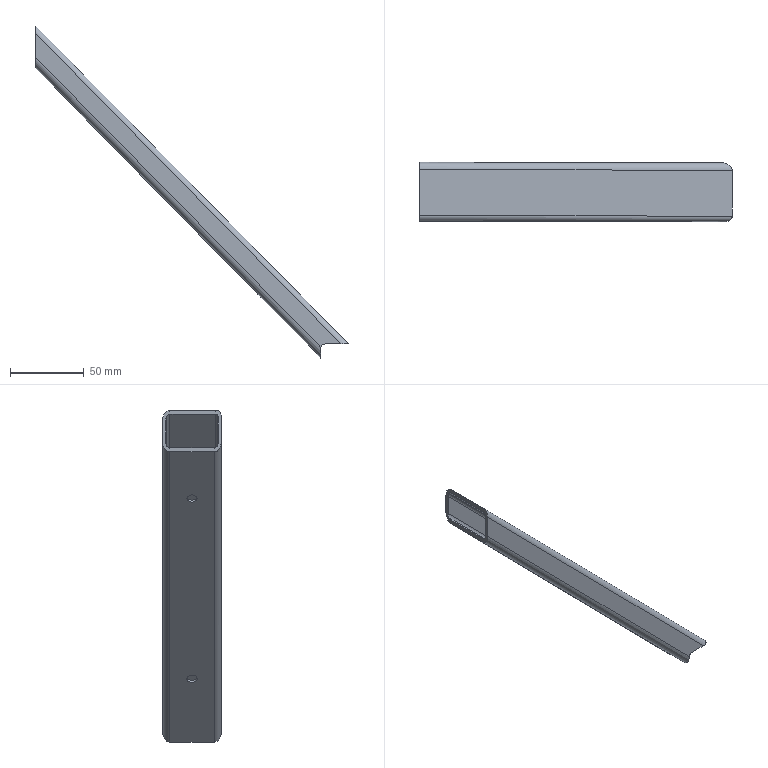Part | NX | features BREP 1 | 1 solid | 31 faces | box 212.69 x 40 x 225.842 mm | volume 60669 mm3 | cylinder 18 | plane 13 | commonest cylinder face diameters 6 x8 7 x4 10 x3 3.502 x2 7.502 x1
STEP:
#1=CARTESIAN_POINT('',(2103.23,-625.419,1266.938));
#2=VERTEX_POINT('',#1);
#3=CARTESIAN_POINT('',(1890.54,-625.419,1483.221));
#4=VERTEX_POINT('',#3);
#5=CARTESIAN_POINT('',(1990.472,-625.419,1381.601));
#6=DIRECTION('',(-0.7012,0.,0.713));
#7=VECTOR('',#6,1000.);
#8=LINE('',#5,#7);
#9=EDGE_CURVE('',#2,#4,#8,.T.);
#10=ORIENTED_EDGE('',*,*,#9,.F.);
#11=CARTESIAN_POINT('',(2103.23,-594.17,1266.938));
#12=VERTEX_POINT('',#11);
#13=CARTESIAN_POINT('',(2103.23,-609.794,1266.938));
#14=DIRECTION('',(0.,-1.,0.));
#15=VECTOR('',#14,1000.);
#16=LINE('',#13,#15);
#17=EDGE_CURVE('',#12,#2,#16,.T.);
#18=ORIENTED_EDGE('',*,*,#17,.F.);
#19=CARTESIAN_POINT('',(1890.54,-594.17,1483.221));
#20=VERTEX_POINT('',#19);
#21=CARTESIAN_POINT('',(1990.472,-594.17,1381.601));
#22=DIRECTION('',(-0.7012,0.,0.713));
#23=VECTOR('',#22,1000.);
#24=LINE('',#21,#23);
#25=EDGE_CURVE('',#12,#20,#24,.T.);
#26=ORIENTED_EDGE('',*,*,#25,.T.);
#27=CARTESIAN_POINT('',(1890.54,-625.419,1483.221));
#28=CARTESIAN_POINT('',(1890.54,-619.169,1483.221));
#29=CARTESIAN_POINT('',(1890.54,-612.919,1483.221));
#30=CARTESIAN_POINT('',(1890.54,-606.67,1483.221));
#31=CARTESIAN_POINT('',(1890.54,-600.42,1483.221));
#32=CARTESIAN_POINT('',(1890.54,-594.17,1483.221));
#33=B_SPLINE_CURVE_WITH_KNOTS('',5,(#27,#28,#29,#30,#31,#32),.UNSPECIFIED.,.F.,.F.,(6,6),(417.921,449.17),.UNSPECIFIED.);
#34=EDGE_CURVE('',#4,#20,#33,.T.);
#35=ORIENTED_EDGE('',*,*,#34,.F.);
#36=EDGE_LOOP('',(#10,#18,#26,#35));
#37=FACE_BOUND('',#36,.T.);
#38=CARTESIAN_POINT('',(2067.213,-625.419,1303.563));
#39=DIRECTION('',(0.713,0.,0.7012));
#40=DIRECTION('',(0.,1.,0.));
#41=AXIS2_PLACEMENT_3D('',#38,#39,#40);
#42=PLANE('',#41);
#43=ADVANCED_FACE('',(#37),#42,.T.);
#44=CARTESIAN_POINT('',(2097.968,-629.17,1266.938));
#45=VERTEX_POINT('',#44);
#46=CARTESIAN_POINT('',(2087.579,-629.17,1266.938));
#47=VERTEX_POINT('',#46);
#48=CARTESIAN_POINT('',(2092.774,-629.17,1266.938));
#49=DIRECTION('',(-1.,0.,0.));
#50=VECTOR('',#49,1000.);
#51=LINE('',#48,#50);
#52=EDGE_CURVE('',#45,#47,#51,.T.);
#53=ORIENTED_EDGE('',*,*,#52,.T.);
#54=CARTESIAN_POINT('',(2087.579,-627.17,1266.938));
#55=VERTEX_POINT('',#54);
#56=CARTESIAN_POINT('',(2087.579,-728.755,1266.938));
#57=DIRECTION('',(0.,1.,0.));
#58=VECTOR('',#57,1000.);
#59=LINE('',#56,#58);
#60=EDGE_CURVE('',#47,#55,#59,.T.);
#61=ORIENTED_EDGE('',*,*,#60,.T.);
#62=CARTESIAN_POINT('',(2097.968,-627.17,1266.938));
#63=VERTEX_POINT('',#62);
#64=CARTESIAN_POINT('',(2092.774,-627.17,1266.938));
#65=DIRECTION('',(-1.,0.,0.));
#66=VECTOR('',#65,1000.);
#67=LINE('',#64,#66);
#68=EDGE_CURVE('',#63,#55,#67,.T.);
#69=ORIENTED_EDGE('',*,*,#68,.F.);
#70=CARTESIAN_POINT('',(2099.705,-626.657,1266.938));
#71=VERTEX_POINT('',#70);
#72=CARTESIAN_POINT('',(2097.968,-627.17,1266.938));
#73=CARTESIAN_POINT('',(2098.602,-627.17,1266.938));
#74=CARTESIAN_POINT('',(2099.227,-626.998,1266.938));
#75=CARTESIAN_POINT('',(2099.705,-626.657,1266.938));
#76=B_SPLINE_CURVE_WITH_KNOTS('',3,(#72,#73,#74,#75),.UNSPECIFIED.,.F.,.F.,(4,4),(0.,1.),.UNSPECIFIED.);
#77=EDGE_CURVE('',#71,#63,#76,.F.);
#78=ORIENTED_EDGE('',*,*,#77,.F.);
#79=CARTESIAN_POINT('',(2100.425,-625.419,1266.938));
#80=VERTEX_POINT('',#79);
#81=CARTESIAN_POINT('',(2099.705,-626.657,1266.938));
#82=CARTESIAN_POINT('',(2100.15,-626.34,1266.938));
#83=CARTESIAN_POINT('',(2100.425,-625.899,1266.938));
#84=CARTESIAN_POINT('',(2100.425,-625.419,1266.938));
#85=B_SPLINE_CURVE_WITH_KNOTS('',3,(#81,#82,#83,#84),.UNSPECIFIED.,.F.,.F.,(4,4),(0.,1.),.UNSPECIFIED.);
#86=EDGE_CURVE('',#80,#71,#85,.F.);
#87=ORIENTED_EDGE('',*,*,#86,.F.);
#88=CARTESIAN_POINT('',(2100.425,-594.17,1266.938));
#89=VERTEX_POINT('',#88);
#90=CARTESIAN_POINT('',(2100.425,-609.794,1266.938));
#91=DIRECTION('',(0.,1.,0.));
#92=VECTOR('',#91,1000.);
#93=LINE('',#90,#92);
#94=EDGE_CURVE('',#80,#89,#93,.T.);
#95=ORIENTED_EDGE('',*,*,#94,.T.);
#96=CARTESIAN_POINT('',(2099.192,-592.049,1266.938));
#97=VERTEX_POINT('',#96);
#98=CARTESIAN_POINT('',(2100.425,-594.17,1266.938));
#99=CARTESIAN_POINT('',(2100.425,-593.338,1266.938));
#100=CARTESIAN_POINT('',(2099.922,-592.569,1266.938));
#101=CARTESIAN_POINT('',(2099.192,-592.049,1266.938));
#102=B_SPLINE_CURVE_WITH_KNOTS('',3,(#98,#99,#100,#101),.UNSPECIFIED.,.F.,.F.,(4,4),(0.,1.),.UNSPECIFIED.);
#103=EDGE_CURVE('',#89,#97,#102,.T.);
#104=ORIENTED_EDGE('',*,*,#103,.T.);
#105=CARTESIAN_POINT('',(2096.217,-591.17,1266.938));
#106=VERTEX_POINT('',#105);
#107=CARTESIAN_POINT('',(2099.192,-592.049,1266.938));
#108=CARTESIAN_POINT('',(2098.37,-591.463,1266.938));
#109=CARTESIAN_POINT('',(2097.283,-591.17,1266.938));
#110=CARTESIAN_POINT('',(2096.217,-591.17,1266.938));
#111=B_SPLINE_CURVE_WITH_KNOTS('',3,(#107,#108,#109,#110),.UNSPECIFIED.,.F.,.F.,(4,4),(0.,1.),.UNSPECIFIED.);
#112=EDGE_CURVE('',#97,#106,#111,.T.);
#113=ORIENTED_EDGE('',*,*,#112,.T.);
#114=CARTESIAN_POINT('',(2087.579,-591.17,1266.938));
#115=VERTEX_POINT('',#114);
#116=CARTESIAN_POINT('',(2091.898,-591.17,1266.938));
#117=DIRECTION('',(-1.,0.,0.));
#118=VECTOR('',#117,1000.);
#119=LINE('',#116,#118);
#120=EDGE_CURVE('',#106,#115,#119,.T.);
#121=ORIENTED_EDGE('',*,*,#120,.T.);
#122=CARTESIAN_POINT('',(2087.579,-589.17,1266.938));
#123=VERTEX_POINT('',#122);
#124=CARTESIAN_POINT('',(2087.579,-708.755,1266.938));
#125=DIRECTION('',(0.,1.,0.));
#126=VECTOR('',#125,1000.);
#127=LINE('',#124,#126);
#128=EDGE_CURVE('',#115,#123,#127,.T.);
#129=ORIENTED_EDGE('',*,*,#128,.T.);
#130=CARTESIAN_POINT('',(2096.217,-589.17,1266.938));
#131=VERTEX_POINT('',#130);
#132=CARTESIAN_POINT('',(2091.898,-589.17,1266.938));
#133=DIRECTION('',(-1.,0.,0.));
#134=VECTOR('',#133,1000.);
#135=LINE('',#132,#134);
#136=EDGE_CURVE('',#131,#123,#135,.T.);
#137=ORIENTED_EDGE('',*,*,#136,.F.);
#138=CARTESIAN_POINT('',(2096.217,-589.17,1266.938));
#139=CARTESIAN_POINT('',(2097.807,-589.17,1266.938));
#140=CARTESIAN_POINT('',(2100.201,-589.72,1266.938));
#141=CARTESIAN_POINT('',(2102.668,-591.822,1266.938));
#142=CARTESIAN_POINT('',(2103.23,-593.382,1266.938));
#143=CARTESIAN_POINT('',(2103.23,-594.17,1266.938));
#144=B_SPLINE_CURVE_WITH_KNOTS('',3,(#138,#139,#140,#141,#142,#143),.UNSPECIFIED.,.F.,.F.,(4,1,1,4),(0.,0.5,0.75,1.),.UNSPECIFIED.);
#145=EDGE_CURVE('',#12,#131,#144,.F.);
#146=ORIENTED_EDGE('',*,*,#145,.F.);
#147=ORIENTED_EDGE('',*,*,#17,.T.);
#148=CARTESIAN_POINT('',(2103.23,-625.419,1266.938));
#149=CARTESIAN_POINT('',(2103.23,-625.838,1266.938));
#150=CARTESIAN_POINT('',(2103.147,-626.257,1266.938));
#151=CARTESIAN_POINT('',(2102.983,-626.653,1266.938));
#152=CARTESIAN_POINT('',(2102.411,-627.575,1266.938));
#153=CARTESIAN_POINT('',(2101.543,-628.249,1266.938));
#154=CARTESIAN_POINT('',(2100.956,-628.566,1266.938));
#155=CARTESIAN_POINT('',(2100.01,-628.927,1266.938));
#156=CARTESIAN_POINT('',(2099.019,-629.107,1266.938));
#157=CARTESIAN_POINT('',(2098.67,-629.149,1266.938));
#158=CARTESIAN_POINT('',(2098.319,-629.17,1266.938));
#159=CARTESIAN_POINT('',(2097.968,-629.17,1266.938));
#160=B_SPLINE_CURVE_WITH_KNOTS('',5,(#148,#149,#150,#151,#152,#153,#154,#155,#156,#157,#158,#159),.UNSPECIFIED.,.F.,.F.,(6,3,3,6),(0.,2.975,7.619,10.108),.UNSPECIFIED.);
#161=EDGE_CURVE('',#2,#45,#160,.T.);
#162=ORIENTED_EDGE('',*,*,#161,.T.);
#163=EDGE_LOOP('',(#53,#61,#69,#78,#87,#95,#104,#113,#121,#129,#137,#146,#147,#162));
#164=FACE_BOUND('',#163,.T.);
#165=CARTESIAN_POINT('',(2104.579,-414.17,1266.938));
#166=DIRECTION('',(0.,0.,1.));
#167=DIRECTION('',(-1.,0.,0.));
#168=AXIS2_PLACEMENT_3D('',#165,#166,#167);
#169=PLANE('',#168);
#170=ADVANCED_FACE('',(#164),#169,.F.);
#171=CARTESIAN_POINT('',(1890.54,-627.17,1477.871));
#172=VERTEX_POINT('',#171);
#173=CARTESIAN_POINT('',(1987.797,-627.17,1378.971));
#174=DIRECTION('',(-0.7012,0.,0.713));
#175=VECTOR('',#174,1000.);
#176=LINE('',#173,#175);
#177=EDGE_CURVE('',#63,#172,#176,.T.);
#178=ORIENTED_EDGE('',*,*,#177,.F.);
#179=ORIENTED_EDGE('',*,*,#68,.T.);
#180=CARTESIAN_POINT('',(2084.625,-627.17,1264.464));
#181=VERTEX_POINT('',#180);
#182=CARTESIAN_POINT('',(2087.579,-627.17,1263.938));
#183=DIRECTION('',(0.,1.,0.));
#184=DIRECTION('',(1.,0.,0.));
#185=AXIS2_PLACEMENT_3D('',#182,#183,#184);
#186=CIRCLE('',#185,3.);
#187=EDGE_CURVE('',#181,#55,#186,.T.);
#188=ORIENTED_EDGE('',*,*,#187,.F.);
#189=CARTESIAN_POINT('',(1890.54,-627.17,1461.828));
#190=VERTEX_POINT('',#189);
#191=CARTESIAN_POINT('',(1979.777,-627.17,1371.084));
#192=DIRECTION('',(-0.7012,0.,0.713));
#193=VECTOR('',#192,1000.);
#194=LINE('',#191,#193);
#195=EDGE_CURVE('',#181,#190,#194,.T.);
#196=ORIENTED_EDGE('',*,*,#195,.T.);
#197=CARTESIAN_POINT('',(1890.54,-627.17,1469.85));
#198=DIRECTION('',(0.,0.,-1.));
#199=VECTOR('',#198,1000.);
#200=LINE('',#197,#199);
#201=EDGE_CURVE('',#172,#190,#200,.T.);
#202=ORIENTED_EDGE('',*,*,#201,.F.);
#203=EDGE_LOOP('',(#178,#179,#188,#196,#202));
#204=FACE_BOUND('',#203,.T.);
#205=CARTESIAN_POINT('',(1839.262,-627.17,1468.228));
#206=DIRECTION('',(0.,-1.,0.));
#207=DIRECTION('',(-0.008377,0.,-1.));
#208=AXIS2_PLACEMENT_3D('',#205,#206,#207);
#209=PLANE('',#208);
#210=ADVANCED_FACE('',(#204),#209,.F.);
#211=ORIENTED_EDGE('',*,*,#77,.T.);
#212=ORIENTED_EDGE('',*,*,#177,.T.);
#213=CARTESIAN_POINT('',(1890.54,-626.657,1479.637));
#214=VERTEX_POINT('',#213);
#215=CARTESIAN_POINT('',(1890.54,-626.657,1479.637));
#216=CARTESIAN_POINT('',(1890.54,-626.995,1479.156));
#217=CARTESIAN_POINT('',(1890.54,-627.17,1478.515));
#218=CARTESIAN_POINT('',(1890.54,-627.17,1477.871));
#219=B_SPLINE_CURVE_WITH_KNOTS('',3,(#215,#216,#217,#218),.UNSPECIFIED.,.F.,.F.,(4,4),(0.,1.),.UNSPECIFIED.);
#220=EDGE_CURVE('',#214,#172,#219,.T.);
#221=ORIENTED_EDGE('',*,*,#220,.F.);
#222=CARTESIAN_POINT('',(1988.68,-626.657,1379.839));
#223=DIRECTION('',(-0.7012,0.,0.713));
#224=VECTOR('',#223,1000.);
#225=LINE('',#222,#224);
#226=EDGE_CURVE('',#71,#214,#225,.T.);
#227=ORIENTED_EDGE('',*,*,#226,.F.);
#228=EDGE_LOOP('',(#211,#212,#221,#227));
#229=FACE_BOUND('',#228,.T.);
#230=CARTESIAN_POINT('',(1987.797,-625.419,1378.971));
#231=DIRECTION('',(-0.7012,0.,0.713));
#232=DIRECTION('',(-0.5042,0.7071,-0.4958));
#233=AXIS2_PLACEMENT_3D('',#230,#231,#232);
#234=CYLINDRICAL_SURFACE('',#233,1.751);
#235=ADVANCED_FACE('',(#229),#234,.F.);
#236=CARTESIAN_POINT('',(1890.54,-625.419,1480.369));
#237=VERTEX_POINT('',#236);
#238=CARTESIAN_POINT('',(1890.54,-625.419,1480.369));
#239=CARTESIAN_POINT('',(1890.54,-625.902,1480.369));
#240=CARTESIAN_POINT('',(1890.54,-626.341,1480.088));
#241=CARTESIAN_POINT('',(1890.54,-626.657,1479.637));
#242=B_SPLINE_CURVE_WITH_KNOTS('',3,(#238,#239,#240,#241),.UNSPECIFIED.,.F.,.F.,(4,4),(0.,1.),.UNSPECIFIED.);
#243=EDGE_CURVE('',#237,#214,#242,.T.);
#244=ORIENTED_EDGE('',*,*,#243,.F.);
#245=CARTESIAN_POINT('',(1995.482,-625.419,1373.654));
#246=DIRECTION('',(-0.7012,0.,0.713));
#247=VECTOR('',#246,1000.);
#248=LINE('',#245,#247);
#249=EDGE_CURVE('',#80,#237,#248,.T.);
#250=ORIENTED_EDGE('',*,*,#249,.F.);
#251=ORIENTED_EDGE('',*,*,#86,.T.);
#252=ORIENTED_EDGE('',*,*,#226,.T.);
#253=EDGE_LOOP('',(#244,#250,#251,#252));
#254=FACE_BOUND('',#253,.T.);
#255=CARTESIAN_POINT('',(1987.797,-625.419,1378.971));
#256=DIRECTION('',(-0.7012,0.,0.713));
#257=DIRECTION('',(0.5042,-0.7071,0.4958));
#258=AXIS2_PLACEMENT_3D('',#255,#256,#257);
#259=CYLINDRICAL_SURFACE('',#258,1.751);
#260=ADVANCED_FACE('',(#254),#259,.F.);
#261=CARTESIAN_POINT('',(1890.54,-594.17,1480.369));
#262=VERTEX_POINT('',#261);
#263=CARTESIAN_POINT('',(1890.54,-609.794,1480.369));
#264=DIRECTION('',(0.,1.,0.));
#265=VECTOR('',#264,1000.);
#266=LINE('',#263,#265);
#267=EDGE_CURVE('',#237,#262,#266,.T.);
#268=ORIENTED_EDGE('',*,*,#267,.T.);
#269=CARTESIAN_POINT('',(1989.046,-594.17,1380.199));
#270=DIRECTION('',(-0.7012,0.,0.713));
#271=VECTOR('',#270,1000.);
#272=LINE('',#269,#271);
#273=EDGE_CURVE('',#89,#262,#272,.T.);
#274=ORIENTED_EDGE('',*,*,#273,.F.);
#275=ORIENTED_EDGE('',*,*,#94,.F.);
#276=ORIENTED_EDGE('',*,*,#249,.T.);
#277=EDGE_LOOP('',(#268,#274,#275,#276));
#278=FACE_BOUND('',#277,.T.);
#279=CARTESIAN_POINT('',(2065.787,-625.419,1302.16));
#280=DIRECTION('',(0.713,0.,0.7012));
#281=DIRECTION('',(0.,1.,0.));
#282=AXIS2_PLACEMENT_3D('',#279,#280,#281);
#283=PLANE('',#282);
#284=ADVANCED_FACE('',(#278),#283,.F.);
#285=ORIENTED_EDGE('',*,*,#103,.F.);
#286=ORIENTED_EDGE('',*,*,#273,.T.);
#287=CARTESIAN_POINT('',(1890.54,-592.049,1479.116));
#288=VERTEX_POINT('',#287);
#289=CARTESIAN_POINT('',(1890.54,-594.17,1480.369));
#290=CARTESIAN_POINT('',(1890.54,-593.953,1480.369));
#291=CARTESIAN_POINT('',(1890.54,-593.737,1480.341));
#292=CARTESIAN_POINT('',(1890.54,-593.524,1480.285));
#293=CARTESIAN_POINT('',(1890.54,-593.051,1480.097));
#294=CARTESIAN_POINT('',(1890.54,-592.631,1479.792));
#295=CARTESIAN_POINT('',(1890.54,-592.414,1479.588));
#296=CARTESIAN_POINT('',(1890.54,-592.22,1479.361));
#297=CARTESIAN_POINT('',(1890.54,-592.049,1479.116));
#298=B_SPLINE_CURVE_WITH_KNOTS('',5,(#289,#290,#291,#292,#293,#294,#295,#296,#297),.UNSPECIFIED.,.F.,.F.,(6,3,6),(0.,1.603,3.714),.UNSPECIFIED.);
#299=EDGE_CURVE('',#262,#288,#298,.T.);
#300=ORIENTED_EDGE('',*,*,#299,.T.);
#301=CARTESIAN_POINT('',(1988.419,-592.049,1379.583));
#302=DIRECTION('',(-0.7012,0.,0.713));
#303=VECTOR('',#302,1000.);
#304=LINE('',#301,#303);
#305=EDGE_CURVE('',#97,#288,#304,.T.);
#306=ORIENTED_EDGE('',*,*,#305,.F.);
#307=EDGE_LOOP('',(#285,#286,#300,#306));
#308=FACE_BOUND('',#307,.T.);
#309=CARTESIAN_POINT('',(1986.907,-594.17,1378.095));
#310=DIRECTION('',(-0.7012,0.,0.713));
#311=DIRECTION('',(-0.5042,-0.7071,-0.4958));
#312=AXIS2_PLACEMENT_3D('',#309,#310,#311);
#313=CYLINDRICAL_SURFACE('',#312,3.);
#314=ADVANCED_FACE('',(#308),#313,.F.);
#315=CARTESIAN_POINT('',(1890.54,-591.17,1476.09));
#316=VERTEX_POINT('',#315);
#317=CARTESIAN_POINT('',(1890.54,-592.049,1479.116));
#318=CARTESIAN_POINT('',(1890.54,-592.02,1479.075));
#319=CARTESIAN_POINT('',(1890.54,-591.992,1479.033));
#320=CARTESIAN_POINT('',(1890.54,-591.964,1478.991));
#321=CARTESIAN_POINT('',(1890.54,-591.706,1478.583));
#322=CARTESIAN_POINT('',(1890.54,-591.504,1478.135));
#323=CARTESIAN_POINT('',(1890.54,-591.368,1477.715));
#324=CARTESIAN_POINT('',(1890.54,-591.239,1477.135));
#325=CARTESIAN_POINT('',(1890.54,-591.184,1476.545));
#326=CARTESIAN_POINT('',(1890.54,-591.175,1476.393));
#327=CARTESIAN_POINT('',(1890.54,-591.17,1476.242));
#328=CARTESIAN_POINT('',(1890.54,-591.17,1476.09));
#329=B_SPLINE_CURVE_WITH_KNOTS('',5,(#317,#318,#319,#320,#321,#322,#323,#324,#325,#326,#327,#328),.UNSPECIFIED.,.F.,.F.,(6,3,3,6),(3.714,4.069,7.114,8.159),.UNSPECIFIED.);
#330=EDGE_CURVE('',#288,#316,#329,.T.);
#331=ORIENTED_EDGE('',*,*,#330,.T.);
#332=CARTESIAN_POINT('',(1993.378,-591.17,1371.514));
#333=DIRECTION('',(-0.7012,0.,0.713));
#334=VECTOR('',#333,1000.);
#335=LINE('',#332,#334);
#336=EDGE_CURVE('',#106,#316,#335,.T.);
#337=ORIENTED_EDGE('',*,*,#336,.F.);
#338=ORIENTED_EDGE('',*,*,#112,.F.);
#339=ORIENTED_EDGE('',*,*,#305,.T.);
#340=EDGE_LOOP('',(#331,#337,#338,#339));
#341=FACE_BOUND('',#340,.T.);
#342=CARTESIAN_POINT('',(1986.907,-594.17,1378.095));
#343=DIRECTION('',(-0.7012,0.,0.713));
#344=DIRECTION('',(0.5042,0.7071,0.4958));
#345=AXIS2_PLACEMENT_3D('',#342,#343,#344);
#346=CYLINDRICAL_SURFACE('',#345,3.);
#347=ADVANCED_FACE('',(#341),#346,.F.);
#348=CARTESIAN_POINT('',(2084.625,-591.17,1264.464));
#349=VERTEX_POINT('',#348);
#350=CARTESIAN_POINT('',(2087.579,-591.17,1263.938));
#351=DIRECTION('',(0.,1.,0.));
#352=DIRECTION('',(1.,0.,0.));
#353=AXIS2_PLACEMENT_3D('',#350,#351,#352);
#354=CIRCLE('',#353,3.);
#355=EDGE_CURVE('',#349,#115,#354,.T.);
#356=ORIENTED_EDGE('',*,*,#355,.T.);
#357=ORIENTED_EDGE('',*,*,#120,.F.);
#358=ORIENTED_EDGE('',*,*,#336,.T.);
#359=CARTESIAN_POINT('',(1890.54,-591.17,1461.828));
#360=VERTEX_POINT('',#359);
#361=CARTESIAN_POINT('',(1890.54,-591.17,1468.959));
#362=DIRECTION('',(0.,0.,-1.));
#363=VECTOR('',#362,1000.);
#364=LINE('',#361,#363);
#365=EDGE_CURVE('',#316,#360,#364,.T.);
#366=ORIENTED_EDGE('',*,*,#365,.T.);
#367=CARTESIAN_POINT('',(1979.777,-591.17,1371.084));
#368=DIRECTION('',(-0.7012,0.,0.713));
#369=VECTOR('',#368,1000.);
#370=LINE('',#367,#369);
#371=EDGE_CURVE('',#349,#360,#370,.T.);
#372=ORIENTED_EDGE('',*,*,#371,.F.);
#373=EDGE_LOOP('',(#356,#357,#358,#366,#372));
#374=FACE_BOUND('',#373,.T.);
#375=CARTESIAN_POINT('',(1839.168,-591.17,1456.98));
#376=DIRECTION('',(0.,1.,0.));
#377=DIRECTION('',(0.008377,0.,1.));
#378=AXIS2_PLACEMENT_3D('',#375,#376,#377);
#379=PLANE('',#378);
#380=ADVANCED_FACE('',(#374),#379,.F.);
#381=CARTESIAN_POINT('',(2084.625,-589.17,1264.464));
#382=VERTEX_POINT('',#381);
#383=CARTESIAN_POINT('',(1890.54,-589.17,1461.828));
#384=VERTEX_POINT('',#383);
#385=CARTESIAN_POINT('',(1979.777,-589.17,1371.084));
#386=DIRECTION('',(-0.7012,0.,0.713));
#387=VECTOR('',#386,1000.);
#388=LINE('',#385,#387);
#389=EDGE_CURVE('',#382,#384,#388,.T.);
#390=ORIENTED_EDGE('',*,*,#389,.T.);
#391=CARTESIAN_POINT('',(1890.54,-589.17,1476.09));
#392=VERTEX_POINT('',#391);
#393=CARTESIAN_POINT('',(1890.54,-589.17,1468.959));
#394=DIRECTION('',(0.,0.,-1.));
#395=VECTOR('',#394,1000.);
#396=LINE('',#393,#395);
#397=EDGE_CURVE('',#392,#384,#396,.T.);
#398=ORIENTED_EDGE('',*,*,#397,.F.);
#399=CARTESIAN_POINT('',(1986.907,-589.17,1378.095));
#400=DIRECTION('',(-0.7012,0.,0.713));
#401=VECTOR('',#400,1000.);
#402=LINE('',#399,#401);
#403=EDGE_CURVE('',#131,#392,#402,.T.);
#404=ORIENTED_EDGE('',*,*,#403,.F.);
#405=ORIENTED_EDGE('',*,*,#136,.T.);
#406=CARTESIAN_POINT('',(2087.579,-589.17,1263.938));
#407=DIRECTION('',(0.,1.,0.));
#408=DIRECTION('',(1.,0.,0.));
#409=AXIS2_PLACEMENT_3D('',#406,#407,#408);
#410=CIRCLE('',#409,3.);
#411=EDGE_CURVE('',#382,#123,#410,.T.);
#412=ORIENTED_EDGE('',*,*,#411,.F.);
#413=EDGE_LOOP('',(#390,#398,#404,#405,#412));
#414=FACE_BOUND('',#413,.T.);
#415=CARTESIAN_POINT('',(1839.168,-589.17,1456.98));
#416=DIRECTION('',(0.,1.,0.));
#417=DIRECTION('',(0.008377,0.,1.));
#418=AXIS2_PLACEMENT_3D('',#415,#416,#417);
#419=PLANE('',#418);
#420=ADVANCED_FACE('',(#414),#419,.T.);
#421=ORIENTED_EDGE('',*,*,#403,.T.);
#422=CARTESIAN_POINT('',(1890.54,-592.854,1482.97));
#423=VERTEX_POINT('',#422);
#424=CARTESIAN_POINT('',(1890.54,-592.854,1482.97));
#425=CARTESIAN_POINT('',(1890.54,-592.47,1482.82));
#426=CARTESIAN_POINT('',(1890.54,-592.105,1482.62));
#427=CARTESIAN_POINT('',(1890.54,-591.767,1482.377));
#428=CARTESIAN_POINT('',(1890.54,-591.081,1481.767));
#429=CARTESIAN_POINT('',(1890.54,-590.53,1481.03));
#430=CARTESIAN_POINT('',(1890.54,-590.267,1480.599));
#431=CARTESIAN_POINT('',(1890.54,-589.711,1479.488));
#432=CARTESIAN_POINT('',(1890.54,-589.37,1478.29));
#433=CARTESIAN_POINT('',(1890.54,-589.237,1477.562));
#434=CARTESIAN_POINT('',(1890.54,-589.17,1476.826));
#435=CARTESIAN_POINT('',(1890.54,-589.17,1476.09));
#436=B_SPLINE_CURVE_WITH_KNOTS('',5,(#424,#425,#426,#427,#428,#429,#430,#431,#432,#433,#434,#435),.UNSPECIFIED.,.F.,.F.,(6,3,3,6),(0.,2.919,6.476,11.688),.UNSPECIFIED.);
#437=EDGE_CURVE('',#423,#392,#436,.T.);
#438=ORIENTED_EDGE('',*,*,#437,.F.);
#439=CARTESIAN_POINT('',(1890.54,-594.17,1483.221));
#440=CARTESIAN_POINT('',(1890.54,-593.723,1483.221));
#441=CARTESIAN_POINT('',(1890.54,-593.285,1483.138));
#442=CARTESIAN_POINT('',(1890.54,-592.854,1482.97));
#443=B_SPLINE_CURVE_WITH_KNOTS('',3,(#439,#440,#441,#442),.UNSPECIFIED.,.F.,.F.,(4,4),(0.,1.),.UNSPECIFIED.);
#444=EDGE_CURVE('',#20,#423,#443,.T.);
#445=ORIENTED_EDGE('',*,*,#444,.F.);
#446=ORIENTED_EDGE('',*,*,#25,.F.);
#447=ORIENTED_EDGE('',*,*,#145,.T.);
#448=EDGE_LOOP('',(#421,#438,#445,#446,#447));
#449=FACE_BOUND('',#448,.T.);
#450=CARTESIAN_POINT('',(1986.907,-594.17,1378.095));
#451=DIRECTION('',(-0.7012,0.,0.713));
#452=DIRECTION('',(0.713,0.,0.7012));
#453=AXIS2_PLACEMENT_3D('',#450,#451,#452);
#454=CYLINDRICAL_SURFACE('',#453,5.);
#455=ADVANCED_FACE('',(#449),#454,.T.);
#456=CARTESIAN_POINT('',(1890.54,-594.17,1482.97));
#457=VERTEX_POINT('',#456);
#458=CARTESIAN_POINT('',(1890.54,-594.17,1482.97));
#459=CARTESIAN_POINT('',(1890.54,-594.17,1483.221));
#460=B_SPLINE_CURVE_WITH_KNOTS('',1,(#458,#459),.UNSPECIFIED.,.F.,.F.,(2,2),(0.,0.2516),.UNSPECIFIED.);
#461=EDGE_CURVE('',#457,#20,#460,.T.);
#462=ORIENTED_EDGE('',*,*,#461,.T.);
#463=ORIENTED_EDGE('',*,*,#444,.T.);
#464=CARTESIAN_POINT('',(1890.54,-593.512,1482.97));
#465=DIRECTION('',(0.,1.,0.));
#466=VECTOR('',#465,1000.);
#467=LINE('',#464,#466);
#468=EDGE_CURVE('',#457,#423,#467,.T.);
#469=ORIENTED_EDGE('',*,*,#468,.F.);
#470=EDGE_LOOP('',(#462,#463,#469));
#471=FACE_BOUND('',#470,.T.);
#472=CARTESIAN_POINT('',(1890.54,-394.17,1483.14));
#473=DIRECTION('',(1.,0.,0.));
#474=DIRECTION('',(0.,0.,-1.));
#475=AXIS2_PLACEMENT_3D('',#472,#473,#474);
#476=PLANE('',#475);
#477=ADVANCED_FACE('',(#471),#476,.F.);
#478=CARTESIAN_POINT('',(1890.54,-626.556,1482.97));
#479=VERTEX_POINT('',#478);
#480=CARTESIAN_POINT('',(1890.54,-626.556,1482.97));
#481=CARTESIAN_POINT('',(1890.54,-626.187,1483.137));
#482=CARTESIAN_POINT('',(1890.54,-625.803,1483.221));
#483=CARTESIAN_POINT('',(1890.54,-625.419,1483.221));
#484=B_SPLINE_CURVE_WITH_KNOTS('',3,(#480,#481,#482,#483),.UNSPECIFIED.,.F.,.F.,(4,4),(0.,1.),.UNSPECIFIED.);
#485=EDGE_CURVE('',#4,#479,#484,.F.);
#486=ORIENTED_EDGE('',*,*,#485,.F.);
#487=ORIENTED_EDGE('',*,*,#34,.T.);
#488=ORIENTED_EDGE('',*,*,#461,.F.);
#489=CARTESIAN_POINT('',(1890.54,-610.363,1482.97));
#490=DIRECTION('',(0.,1.,0.));
#491=VECTOR('',#490,1000.);
#492=LINE('',#489,#491);
#493=EDGE_CURVE('',#479,#457,#492,.T.);
#494=ORIENTED_EDGE('',*,*,#493,.F.);
#495=EDGE_LOOP('',(#486,#487,#488,#494));
#496=FACE_BOUND('',#495,.T.);
#497=CARTESIAN_POINT('',(1890.54,-414.17,1483.14));
#498=DIRECTION('',(1.,0.,0.));
#499=DIRECTION('',(0.,0.,-1.));
#500=AXIS2_PLACEMENT_3D('',#497,#498,#499);
#501=PLANE('',#500);
#502=ADVANCED_FACE('',(#496),#501,.F.);
#503=ORIENTED_EDGE('',*,*,#9,.T.);
#504=ORIENTED_EDGE('',*,*,#485,.T.);
#505=CARTESIAN_POINT('',(1890.54,-629.17,1477.871));
#506=VERTEX_POINT('',#505);
#507=CARTESIAN_POINT('',(1890.54,-626.556,1482.97));
#508=CARTESIAN_POINT('',(1890.54,-626.8,1482.859));
#509=CARTESIAN_POINT('',(1890.54,-627.032,1482.721));
#510=CARTESIAN_POINT('',(1890.54,-627.25,1482.56));
#511=CARTESIAN_POINT('',(1890.54,-627.779,1482.088));
#512=CARTESIAN_POINT('',(1890.54,-628.2,1481.514));
#513=CARTESIAN_POINT('',(1890.54,-628.421,1481.132));
#514=CARTESIAN_POINT('',(1890.54,-628.814,1480.278));
#515=CARTESIAN_POINT('',(1890.54,-629.047,1479.365));
#516=CARTESIAN_POINT('',(1890.54,-629.129,1478.87));
#517=CARTESIAN_POINT('',(1890.54,-629.17,1478.371));
#518=CARTESIAN_POINT('',(1890.54,-629.17,1477.871));
#519=B_SPLINE_CURVE_WITH_KNOTS('',5,(#507,#508,#509,#510,#511,#512,#513,#514,#515,#516,#517,#518),.UNSPECIFIED.,.F.,.F.,(6,3,3,6),(0.,1.902,5.003,8.54),.UNSPECIFIED.);
#520=EDGE_CURVE('',#479,#506,#519,.T.);
#521=ORIENTED_EDGE('',*,*,#520,.T.);
#522=CARTESIAN_POINT('',(1994.254,-629.17,1372.405));
#523=DIRECTION('',(-0.7012,0.,0.713));
#524=VECTOR('',#523,1000.);
#525=LINE('',#522,#524);
#526=EDGE_CURVE('',#45,#506,#525,.T.);
#527=ORIENTED_EDGE('',*,*,#526,.F.);
#528=ORIENTED_EDGE('',*,*,#161,.F.);
#529=EDGE_LOOP('',(#503,#504,#521,#527,#528));
#530=FACE_BOUND('',#529,.T.);
#531=CARTESIAN_POINT('',(1987.797,-625.419,1378.971));
#532=DIRECTION('',(-0.7012,0.,0.713));
#533=DIRECTION('',(0.,-1.,0.));
#534=AXIS2_PLACEMENT_3D('',#531,#532,#533);
#535=CYLINDRICAL_SURFACE('',#534,3.751);
#536=ADVANCED_FACE('',(#530),#535,.T.);
#537=ORIENTED_EDGE('',*,*,#526,.T.);
#538=CARTESIAN_POINT('',(1890.54,-629.17,1461.828));
#539=VERTEX_POINT('',#538);
#540=CARTESIAN_POINT('',(1890.54,-629.17,1469.85));
#541=DIRECTION('',(0.,0.,-1.));
#542=VECTOR('',#541,1000.);
#543=LINE('',#540,#542);
#544=EDGE_CURVE('',#506,#539,#543,.T.);
#545=ORIENTED_EDGE('',*,*,#544,.T.);
#546=CARTESIAN_POINT('',(2084.625,-629.17,1264.464));
#547=VERTEX_POINT('',#546);
#548=CARTESIAN_POINT('',(1979.777,-629.17,1371.084));
#549=DIRECTION('',(-0.7012,0.,0.713));
#550=VECTOR('',#549,1000.);
#551=LINE('',#548,#550);
#552=EDGE_CURVE('',#547,#539,#551,.T.);
#553=ORIENTED_EDGE('',*,*,#552,.F.);
#554=CARTESIAN_POINT('',(2087.579,-629.17,1263.938));
#555=DIRECTION('',(0.,1.,0.));
#556=DIRECTION('',(1.,0.,0.));
#557=AXIS2_PLACEMENT_3D('',#554,#555,#556);
#558=CIRCLE('',#557,3.);
#559=EDGE_CURVE('',#547,#47,#558,.T.);
#560=ORIENTED_EDGE('',*,*,#559,.T.);
#561=ORIENTED_EDGE('',*,*,#52,.F.);
#562=EDGE_LOOP('',(#537,#545,#553,#560,#561));
#563=FACE_BOUND('',#562,.T.);
#564=CARTESIAN_POINT('',(1839.262,-629.17,1468.228));
#565=DIRECTION('',(0.,-1.,0.));
#566=DIRECTION('',(-0.008377,0.,-1.));
#567=AXIS2_PLACEMENT_3D('',#564,#565,#566);
#568=PLANE('',#567);
#569=ADVANCED_FACE('',(#563),#568,.T.);
#570=CARTESIAN_POINT('',(2043.704,-605.67,1301.798));
#571=VERTEX_POINT('',#570);
#572=CARTESIAN_POINT('',(2042.279,-605.67,1300.395));
#573=VERTEX_POINT('',#572);
#574=CARTESIAN_POINT('',(2042.278,-605.67,1300.396));
#575=DIRECTION('',(0.713,0.,0.7012));
#576=VECTOR('',#575,1000.);
#577=LINE('',#574,#576);
#578=EDGE_CURVE('',#571,#573,#577,.F.);
#579=ORIENTED_EDGE('',*,*,#578,.F.);
#580=CARTESIAN_POINT('',(2043.705,-612.67,1301.797));
#581=VERTEX_POINT('',#580);
#582=CARTESIAN_POINT('',(2043.704,-612.67,1301.797));
#583=CARTESIAN_POINT('',(2043.053,-612.67,1302.459));
#584=CARTESIAN_POINT('',(2041.786,-611.912,1303.748));
#585=CARTESIAN_POINT('',(2040.982,-609.17,1304.566));
#586=CARTESIAN_POINT('',(2041.786,-606.428,1303.748));
#587=CARTESIAN_POINT('',(2043.053,-605.67,1302.46));
#588=CARTESIAN_POINT('',(2043.704,-605.67,1301.798));
#589=B_SPLINE_CURVE_WITH_KNOTS('',3,(#582,#583,#584,#585,#586,#587,#588),.UNSPECIFIED.,.F.,.F.,(4,1,1,1,4),(0.,0.25,0.5,0.75,0.9999),.UNSPECIFIED.);
#590=EDGE_CURVE('',#571,#581,#589,.F.);
#591=ORIENTED_EDGE('',*,*,#590,.T.);
#592=CARTESIAN_POINT('',(2042.278,-612.67,1300.396));
#593=VERTEX_POINT('',#592);
#594=CARTESIAN_POINT('',(2042.278,-612.67,1300.396));
#595=DIRECTION('',(0.713,0.,0.7012));
#596=VECTOR('',#595,1000.);
#597=LINE('',#594,#596);
#598=EDGE_CURVE('',#581,#593,#597,.F.);
#599=ORIENTED_EDGE('',*,*,#598,.T.);
#600=CARTESIAN_POINT('',(2042.278,-605.67,1300.395));
#601=CARTESIAN_POINT('',(2041.628,-605.67,1301.057));
#602=CARTESIAN_POINT('',(2040.36,-606.428,1302.345));
#603=CARTESIAN_POINT('',(2039.556,-609.169,1303.163));
#604=CARTESIAN_POINT('',(2040.36,-611.912,1302.346));
#605=CARTESIAN_POINT('',(2041.626,-612.67,1301.058));
#606=CARTESIAN_POINT('',(2042.278,-612.67,1300.396));
#607=B_SPLINE_CURVE_WITH_KNOTS('',3,(#600,#601,#602,#603,#604,#605,#606),.UNSPECIFIED.,.F.,.F.,(4,1,1,1,4),(0.,0.25,0.5,0.75,0.9999),.UNSPECIFIED.);
#608=EDGE_CURVE('',#573,#593,#607,.T.);
#609=ORIENTED_EDGE('',*,*,#608,.F.);
#610=EDGE_LOOP('',(#579,#591,#599,#609));
#611=FACE_BOUND('',#610,.T.);
#612=CARTESIAN_POINT('',(-4275992.175,-609.17,-4205648.762));
#613=DIRECTION('',(0.713,0.,0.7012));
#614=DIRECTION('',(0.7012,0.,-0.713));
#615=AXIS2_PLACEMENT_3D('',#612,#613,#614);
#616=CYLINDRICAL_SURFACE('',#615,3.5);
#617=ADVANCED_FACE('',(#611),#616,.F.);
#618=ORIENTED_EDGE('',*,*,#598,.F.);
#619=CARTESIAN_POINT('',(2043.704,-605.67,1301.797));
#620=CARTESIAN_POINT('',(2044.355,-605.67,1301.136));
#621=CARTESIAN_POINT('',(2045.622,-606.428,1299.847));
#622=CARTESIAN_POINT('',(2046.426,-609.17,1299.029));
#623=CARTESIAN_POINT('',(2045.622,-611.912,1299.847));
#624=CARTESIAN_POINT('',(2044.356,-612.67,1301.135));
#625=CARTESIAN_POINT('',(2043.705,-612.67,1301.797));
#626=B_SPLINE_CURVE_WITH_KNOTS('',3,(#619,#620,#621,#622,#623,#624,#625),.UNSPECIFIED.,.F.,.F.,(4,1,1,1,4),(0.,0.25,0.5,0.75,0.9999),.UNSPECIFIED.);
#627=EDGE_CURVE('',#581,#571,#626,.F.);
#628=ORIENTED_EDGE('',*,*,#627,.T.);
#629=ORIENTED_EDGE('',*,*,#578,.T.);
#630=CARTESIAN_POINT('',(2042.278,-612.67,1300.395));
#631=CARTESIAN_POINT('',(2042.929,-612.67,1299.734));
#632=CARTESIAN_POINT('',(2044.196,-611.912,1298.445));
#633=CARTESIAN_POINT('',(2045.,-609.171,1297.627));
#634=CARTESIAN_POINT('',(2044.197,-606.428,1298.444));
#635=CARTESIAN_POINT('',(2042.93,-605.67,1299.732));
#636=CARTESIAN_POINT('',(2042.279,-605.67,1300.395));
#637=B_SPLINE_CURVE_WITH_KNOTS('',3,(#630,#631,#632,#633,#634,#635,#636),.UNSPECIFIED.,.F.,.F.,(4,1,1,1,4),(0.,0.25,0.5,0.75,0.9999),.UNSPECIFIED.);
#638=EDGE_CURVE('',#593,#573,#637,.T.);
#639=ORIENTED_EDGE('',*,*,#638,.F.);
#640=EDGE_LOOP('',(#618,#628,#629,#639));
#641=FACE_BOUND('',#640,.T.);
#642=CARTESIAN_POINT('',(-4275992.175,-609.17,-4205648.762));
#643=DIRECTION('',(0.713,0.,0.7012));
#644=DIRECTION('',(0.7012,0.,-0.713));
#645=AXIS2_PLACEMENT_3D('',#642,#643,#644);
#646=CYLINDRICAL_SURFACE('',#645,3.5);
#647=ADVANCED_FACE('',(#641),#646,.F.);
#648=CARTESIAN_POINT('',(1921.679,-612.67,1423.032));
#649=VERTEX_POINT('',#648);
#650=CARTESIAN_POINT('',(1923.105,-612.67,1424.435));
#651=VERTEX_POINT('',#650);
#652=CARTESIAN_POINT('',(1921.67,-612.67,1423.023));
#653=DIRECTION('',(0.713,0.,0.7012));
#654=VECTOR('',#653,1000.);
#655=LINE('',#652,#654);
#656=EDGE_CURVE('',#649,#651,#655,.T.);
#657=ORIENTED_EDGE('',*,*,#656,.T.);
#658=CARTESIAN_POINT('',(1923.105,-605.67,1424.435));
#659=VERTEX_POINT('',#658);
#660=CARTESIAN_POINT('',(1923.105,-605.67,1424.435));
#661=CARTESIAN_POINT('',(1923.749,-605.67,1423.78));
#662=CARTESIAN_POINT('',(1925.026,-606.427,1422.481));
#663=CARTESIAN_POINT('',(1925.825,-609.17,1421.668));
#664=CARTESIAN_POINT('',(1925.026,-611.913,1422.481));
#665=CARTESIAN_POINT('',(1923.75,-612.67,1423.779));
#666=CARTESIAN_POINT('',(1923.105,-612.67,1424.435));
#667=B_SPLINE_CURVE_WITH_KNOTS('',3,(#660,#661,#662,#663,#664,#665,#666),.UNSPECIFIED.,.F.,.F.,(4,1,1,1,4),(0.,0.25,0.5,0.75,1.),.UNSPECIFIED.);
#668=EDGE_CURVE('',#659,#651,#667,.T.);
#669=ORIENTED_EDGE('',*,*,#668,.F.);
#670=CARTESIAN_POINT('',(1921.679,-605.67,1423.032));
#671=VERTEX_POINT('',#670);
#672=CARTESIAN_POINT('',(1921.67,-605.67,1423.023));
#673=DIRECTION('',(0.713,0.,0.7012));
#674=VECTOR('',#673,1000.);
#675=LINE('',#672,#674);
#676=EDGE_CURVE('',#671,#659,#675,.T.);
#677=ORIENTED_EDGE('',*,*,#676,.F.);
#678=CARTESIAN_POINT('',(1921.679,-609.17,1423.032));
#679=DIRECTION('',(-0.713,0.,-0.7012));
#680=DIRECTION('',(-0.7012,0.,0.713));
#681=AXIS2_PLACEMENT_3D('',#678,#679,#680);
#682=CIRCLE('',#681,3.5);
#683=EDGE_CURVE('',#671,#649,#682,.T.);
#684=ORIENTED_EDGE('',*,*,#683,.T.);
#685=EDGE_LOOP('',(#657,#669,#677,#684));
#686=FACE_BOUND('',#685,.T.);
#687=CARTESIAN_POINT('',(1921.67,-609.17,1423.023));
#688=DIRECTION('',(0.713,0.,0.7012));
#689=DIRECTION('',(0.,-1.,0.));
#690=AXIS2_PLACEMENT_3D('',#687,#688,#689);
#691=CYLINDRICAL_SURFACE('',#690,3.5);
#692=ADVANCED_FACE('',(#686),#691,.F.);
#693=ORIENTED_EDGE('',*,*,#676,.T.);
#694=CARTESIAN_POINT('',(1923.105,-612.67,1424.435));
#695=CARTESIAN_POINT('',(1922.461,-612.67,1425.09));
#696=CARTESIAN_POINT('',(1921.183,-611.913,1426.389));
#697=CARTESIAN_POINT('',(1920.384,-609.17,1427.201));
#698=CARTESIAN_POINT('',(1921.184,-606.427,1426.388));
#699=CARTESIAN_POINT('',(1922.46,-605.67,1425.091));
#700=CARTESIAN_POINT('',(1923.105,-605.67,1424.435));
#701=B_SPLINE_CURVE_WITH_KNOTS('',3,(#694,#695,#696,#697,#698,#699,#700),.UNSPECIFIED.,.F.,.F.,(4,1,1,1,4),(0.,0.25,0.5,0.75,1.),.UNSPECIFIED.);
#702=EDGE_CURVE('',#651,#659,#701,.T.);
#703=ORIENTED_EDGE('',*,*,#702,.F.);
#704=ORIENTED_EDGE('',*,*,#656,.F.);
#705=CARTESIAN_POINT('',(1921.679,-609.17,1423.032));
#706=DIRECTION('',(-0.713,0.,-0.7012));
#707=DIRECTION('',(-0.7012,0.,0.713));
#708=AXIS2_PLACEMENT_3D('',#705,#706,#707);
#709=CIRCLE('',#708,3.5);
#710=EDGE_CURVE('',#649,#671,#709,.T.);
#711=ORIENTED_EDGE('',*,*,#710,.T.);
#712=EDGE_LOOP('',(#693,#703,#704,#711));
#713=FACE_BOUND('',#712,.T.);
#714=CARTESIAN_POINT('',(1921.67,-609.17,1423.023));
#715=DIRECTION('',(0.713,0.,0.7012));
#716=DIRECTION('',(0.,1.,0.));
#717=AXIS2_PLACEMENT_3D('',#714,#715,#716);
#718=CYLINDRICAL_SURFACE('',#717,3.5);
#719=ADVANCED_FACE('',(#713),#718,.F.);
#720=CARTESIAN_POINT('',(1890.54,-624.17,1454.697));
#721=VERTEX_POINT('',#720);
#722=CARTESIAN_POINT('',(1890.54,-624.17,1454.697));
#723=CARTESIAN_POINT('',(1890.54,-624.966,1454.697));
#724=CARTESIAN_POINT('',(1890.54,-626.54,1455.282));
#725=CARTESIAN_POINT('',(1890.54,-628.629,1457.803));
#726=CARTESIAN_POINT('',(1890.54,-629.17,1460.22));
#727=CARTESIAN_POINT('',(1890.54,-629.17,1461.828));
#728=B_SPLINE_CURVE_WITH_KNOTS('',3,(#722,#723,#724,#725,#726,#727),.UNSPECIFIED.,.F.,.F.,(4,1,1,4),(0.,0.25,0.5,1.),.UNSPECIFIED.);
#729=EDGE_CURVE('',#721,#539,#728,.T.);
#730=ORIENTED_EDGE('',*,*,#729,.F.);
#731=CARTESIAN_POINT('',(2084.579,-624.17,1257.38));
#732=VERTEX_POINT('',#731);
#733=CARTESIAN_POINT('',(1987.559,-624.17,1356.038));
#734=DIRECTION('',(-0.7012,0.,0.713));
#735=VECTOR('',#734,1000.);
#736=LINE('',#733,#735);
#737=EDGE_CURVE('',#732,#721,#736,.T.);
#738=ORIENTED_EDGE('',*,*,#737,.F.);
#739=CARTESIAN_POINT('',(2084.579,-629.154,1263.938));
#740=VERTEX_POINT('',#739);
#741=CARTESIAN_POINT('',(2084.579,-629.154,1263.938));
#742=CARTESIAN_POINT('',(2084.579,-629.11,1263.168));
#743=CARTESIAN_POINT('',(2084.579,-628.936,1262.096));
#744=CARTESIAN_POINT('',(2084.579,-628.383,1260.606));
#745=CARTESIAN_POINT('',(2084.579,-627.884,1259.677));
#746=CARTESIAN_POINT('',(2084.579,-627.128,1258.704));
#747=CARTESIAN_POINT('',(2084.579,-626.06,1257.795));
#748=CARTESIAN_POINT('',(2084.579,-624.919,1257.38));
#749=CARTESIAN_POINT('',(2084.579,-624.17,1257.38));
#750=B_SPLINE_CURVE_WITH_KNOTS('',3,(#741,#742,#743,#744,#745,#746,#747,#748,#749),.UNSPECIFIED.,.F.,.F.,(4,1,1,1,1,1,4),(0.,0.25,0.375,0.5,0.625,0.75,1.),.UNSPECIFIED.);
#751=EDGE_CURVE('',#732,#740,#750,.F.);
#752=ORIENTED_EDGE('',*,*,#751,.T.);
#753=CARTESIAN_POINT('',(2084.579,-629.154,1263.938));
#754=CARTESIAN_POINT('',(2084.579,-629.164,1264.115));
#755=CARTESIAN_POINT('',(2084.594,-629.17,1264.29));
#756=CARTESIAN_POINT('',(2084.625,-629.17,1264.464));
#757=B_SPLINE_CURVE_WITH_KNOTS('',3,(#753,#754,#755,#756),.UNSPECIFIED.,.F.,.F.,(4,4),(0.,1.),.UNSPECIFIED.);
#758=EDGE_CURVE('',#740,#547,#757,.T.);
#759=ORIENTED_EDGE('',*,*,#758,.T.);
#760=ORIENTED_EDGE('',*,*,#552,.T.);
#761=EDGE_LOOP('',(#730,#738,#752,#759,#760));
#762=FACE_BOUND('',#761,.T.);
#763=CARTESIAN_POINT('',(1979.777,-624.17,1371.084));
#764=DIRECTION('',(-0.7012,0.,0.713));
#765=DIRECTION('',(-0.713,0.,-0.7012));
#766=AXIS2_PLACEMENT_3D('',#763,#764,#765);
#767=CYLINDRICAL_SURFACE('',#766,5.);
#768=ADVANCED_FACE('',(#762),#767,.T.);
#769=ORIENTED_EDGE('',*,*,#60,.F.);
#770=ORIENTED_EDGE('',*,*,#559,.F.);
#771=ORIENTED_EDGE('',*,*,#758,.F.);
#772=CARTESIAN_POINT('',(2084.579,-627.143,1263.938));
#773=VERTEX_POINT('',#772);
#774=CARTESIAN_POINT('',(2084.579,-628.148,1263.938));
#775=DIRECTION('',(0.,1.,0.));
#776=VECTOR('',#775,1000.);
#777=LINE('',#774,#776);
#778=EDGE_CURVE('',#740,#773,#777,.T.);
#779=ORIENTED_EDGE('',*,*,#778,.T.);
#780=CARTESIAN_POINT('',(2084.579,-627.143,1263.938));
#781=CARTESIAN_POINT('',(2084.579,-627.161,1264.128));
#782=CARTESIAN_POINT('',(2084.597,-627.17,1264.304));
#783=CARTESIAN_POINT('',(2084.625,-627.17,1264.464));
#784=B_SPLINE_CURVE_WITH_KNOTS('',3,(#780,#781,#782,#783),.UNSPECIFIED.,.F.,.F.,(4,4),(0.,1.),.UNSPECIFIED.);
#785=EDGE_CURVE('',#773,#181,#784,.T.);
#786=ORIENTED_EDGE('',*,*,#785,.T.);
#787=ORIENTED_EDGE('',*,*,#187,.T.);
#788=EDGE_LOOP('',(#769,#770,#771,#779,#786,#787));
#789=FACE_BOUND('',#788,.T.);
#790=CARTESIAN_POINT('',(2087.579,-728.755,1263.938));
#791=DIRECTION('',(0.,1.,0.));
#792=DIRECTION('',(-1.,0.,0.));
#793=AXIS2_PLACEMENT_3D('',#790,#791,#792);
#794=CYLINDRICAL_SURFACE('',#793,3.);
#795=ADVANCED_FACE('',(#789),#794,.F.);
#796=CARTESIAN_POINT('',(1890.54,-594.17,1457.55));
#797=VERTEX_POINT('',#796);
#798=CARTESIAN_POINT('',(1890.54,-592.049,1458.803));
#799=VERTEX_POINT('',#798);
#800=CARTESIAN_POINT('',(1890.54,-594.17,1457.55));
#801=CARTESIAN_POINT('',(1890.54,-593.953,1457.55));
#802=CARTESIAN_POINT('',(1890.54,-593.737,1457.578));
#803=CARTESIAN_POINT('',(1890.54,-593.524,1457.633));
#804=CARTESIAN_POINT('',(1890.54,-593.051,1457.821));
#805=CARTESIAN_POINT('',(1890.54,-592.631,1458.126));
#806=CARTESIAN_POINT('',(1890.54,-592.414,1458.331));
#807=CARTESIAN_POINT('',(1890.54,-592.22,1458.558));
#808=CARTESIAN_POINT('',(1890.54,-592.049,1458.803));
#809=B_SPLINE_CURVE_WITH_KNOTS('',5,(#800,#801,#802,#803,#804,#805,#806,#807,#808),.UNSPECIFIED.,.F.,.F.,(6,3,6),(0.,1.603,3.714),.UNSPECIFIED.);
#810=EDGE_CURVE('',#797,#799,#809,.T.);
#811=ORIENTED_EDGE('',*,*,#810,.F.);
#812=CARTESIAN_POINT('',(2084.579,-594.17,1260.232));
#813=VERTEX_POINT('',#812);
#814=CARTESIAN_POINT('',(1987.559,-594.17,1358.891));
#815=DIRECTION('',(-0.7012,0.,0.713));
#816=VECTOR('',#815,1000.);
#817=LINE('',#814,#816);
#818=EDGE_CURVE('',#813,#797,#817,.T.);
#819=ORIENTED_EDGE('',*,*,#818,.F.);
#820=CARTESIAN_POINT('',(2084.579,-592.049,1261.485));
#821=VERTEX_POINT('',#820);
#822=CARTESIAN_POINT('',(2084.579,-594.17,1260.232));
#823=CARTESIAN_POINT('',(2084.579,-593.953,1260.232));
#824=CARTESIAN_POINT('',(2084.579,-593.737,1260.26));
#825=CARTESIAN_POINT('',(2084.579,-593.524,1260.316));
#826=CARTESIAN_POINT('',(2084.579,-593.051,1260.504));
#827=CARTESIAN_POINT('',(2084.579,-592.631,1260.809));
#828=CARTESIAN_POINT('',(2084.579,-592.414,1261.013));
#829=CARTESIAN_POINT('',(2084.579,-592.22,1261.241));
#830=CARTESIAN_POINT('',(2084.579,-592.049,1261.485));
#831=B_SPLINE_CURVE_WITH_KNOTS('',5,(#822,#823,#824,#825,#826,#827,#828,#829,#830),.UNSPECIFIED.,.F.,.F.,(6,3,6),(0.,1.598,3.703),.UNSPECIFIED.);
#832=EDGE_CURVE('',#813,#821,#831,.T.);
#833=ORIENTED_EDGE('',*,*,#832,.T.);
#834=CARTESIAN_POINT('',(1978.264,-592.049,1369.596));
#835=DIRECTION('',(-0.7012,0.,0.713));
#836=VECTOR('',#835,1000.);
#837=LINE('',#834,#836);
#838=EDGE_CURVE('',#821,#799,#837,.T.);
#839=ORIENTED_EDGE('',*,*,#838,.T.);
#840=EDGE_LOOP('',(#811,#819,#833,#839));
#841=FACE_BOUND('',#840,.T.);
#842=CARTESIAN_POINT('',(1979.777,-594.17,1371.084));
#843=DIRECTION('',(-0.7012,0.,0.713));
#844=DIRECTION('',(-0.5042,0.7071,-0.4958));
#845=AXIS2_PLACEMENT_3D('',#842,#843,#844);
#846=CYLINDRICAL_SURFACE('',#845,3.);
#847=ADVANCED_FACE('',(#841),#846,.F.);
#848=CARTESIAN_POINT('',(2084.579,-591.197,1263.938));
#849=VERTEX_POINT('',#848);
#850=CARTESIAN_POINT('',(2084.579,-592.049,1261.485));
#851=CARTESIAN_POINT('',(2084.579,-592.02,1261.527));
#852=CARTESIAN_POINT('',(2084.579,-591.992,1261.568));
#853=CARTESIAN_POINT('',(2084.579,-591.964,1261.61));
#854=CARTESIAN_POINT('',(2084.579,-591.686,1262.049));
#855=CARTESIAN_POINT('',(2084.579,-591.474,1262.533));
#856=CARTESIAN_POINT('',(2084.579,-591.334,1262.992));
#857=CARTESIAN_POINT('',(2084.579,-591.242,1263.462));
#858=CARTESIAN_POINT('',(2084.579,-591.197,1263.938));
#859=B_SPLINE_CURVE_WITH_KNOTS('',5,(#850,#851,#852,#853,#854,#855,#856,#857,#858),.UNSPECIFIED.,.F.,.F.,(6,3,6),(3.703,4.056,7.346),.UNSPECIFIED.);
#860=EDGE_CURVE('',#821,#849,#859,.T.);
#861=ORIENTED_EDGE('',*,*,#860,.T.);
#862=CARTESIAN_POINT('',(2084.579,-591.197,1263.938));
#863=CARTESIAN_POINT('',(2084.579,-591.18,1264.116));
#864=CARTESIAN_POINT('',(2084.594,-591.17,1264.291));
#865=CARTESIAN_POINT('',(2084.625,-591.17,1264.464));
#866=B_SPLINE_CURVE_WITH_KNOTS('',3,(#862,#863,#864,#865),.UNSPECIFIED.,.F.,.F.,(4,4),(0.,1.),.UNSPECIFIED.);
#867=EDGE_CURVE('',#849,#349,#866,.T.);
#868=ORIENTED_EDGE('',*,*,#867,.T.);
#869=ORIENTED_EDGE('',*,*,#371,.T.);
#870=CARTESIAN_POINT('',(1890.54,-592.049,1458.803));
#871=CARTESIAN_POINT('',(1890.54,-592.02,1458.844));
#872=CARTESIAN_POINT('',(1890.54,-591.992,1458.886));
#873=CARTESIAN_POINT('',(1890.54,-591.964,1458.928));
#874=CARTESIAN_POINT('',(1890.54,-591.706,1459.335));
#875=CARTESIAN_POINT('',(1890.54,-591.504,1459.783));
#876=CARTESIAN_POINT('',(1890.54,-591.368,1460.203));
#877=CARTESIAN_POINT('',(1890.54,-591.239,1460.783));
#878=CARTESIAN_POINT('',(1890.54,-591.184,1461.374));
#879=CARTESIAN_POINT('',(1890.54,-591.175,1461.525));
#880=CARTESIAN_POINT('',(1890.54,-591.17,1461.677));
#881=CARTESIAN_POINT('',(1890.54,-591.17,1461.828));
#882=B_SPLINE_CURVE_WITH_KNOTS('',5,(#870,#871,#872,#873,#874,#875,#876,#877,#878,#879,#880,#881),.UNSPECIFIED.,.F.,.F.,(6,3,3,6),(3.714,4.069,7.114,8.159),.UNSPECIFIED.);
#883=EDGE_CURVE('',#799,#360,#882,.T.);
#884=ORIENTED_EDGE('',*,*,#883,.F.);
#885=ORIENTED_EDGE('',*,*,#838,.F.);
#886=EDGE_LOOP('',(#861,#868,#869,#884,#885));
#887=FACE_BOUND('',#886,.T.);
#888=CARTESIAN_POINT('',(1979.777,-594.17,1371.084));
#889=DIRECTION('',(-0.7012,0.,0.713));
#890=DIRECTION('',(0.5042,-0.7071,0.4958));
#891=AXIS2_PLACEMENT_3D('',#888,#889,#890);
#892=CYLINDRICAL_SURFACE('',#891,3.);
#893=ADVANCED_FACE('',(#887),#892,.F.);
#894=CARTESIAN_POINT('',(2084.579,-589.186,1263.938));
#895=VERTEX_POINT('',#894);
#896=CARTESIAN_POINT('',(2084.579,-590.192,1263.938));
#897=DIRECTION('',(0.,1.,0.));
#898=VECTOR('',#897,1000.);
#899=LINE('',#896,#898);
#900=EDGE_CURVE('',#849,#895,#899,.T.);
#901=ORIENTED_EDGE('',*,*,#900,.T.);
#902=CARTESIAN_POINT('',(2084.579,-589.186,1263.938));
#903=CARTESIAN_POINT('',(2084.579,-589.175,1264.129));
#904=CARTESIAN_POINT('',(2084.597,-589.17,1264.305));
#905=CARTESIAN_POINT('',(2084.625,-589.17,1264.464));
#906=B_SPLINE_CURVE_WITH_KNOTS('',3,(#902,#903,#904,#905),.UNSPECIFIED.,.F.,.F.,(4,4),(0.,1.),.UNSPECIFIED.);
#907=EDGE_CURVE('',#895,#382,#906,.T.);
#908=ORIENTED_EDGE('',*,*,#907,.T.);
#909=ORIENTED_EDGE('',*,*,#411,.T.);
#910=ORIENTED_EDGE('',*,*,#128,.F.);
#911=ORIENTED_EDGE('',*,*,#355,.F.);
#912=ORIENTED_EDGE('',*,*,#867,.F.);
#913=EDGE_LOOP('',(#901,#908,#909,#910,#911,#912));
#914=FACE_BOUND('',#913,.T.);
#915=CARTESIAN_POINT('',(2087.579,-708.755,1263.938));
#916=DIRECTION('',(0.,1.,0.));
#917=DIRECTION('',(-1.,0.,0.));
#918=AXIS2_PLACEMENT_3D('',#915,#916,#917);
#919=CYLINDRICAL_SURFACE('',#918,3.);
#920=ADVANCED_FACE('',(#914),#919,.F.);
#921=CARTESIAN_POINT('',(2084.579,-594.17,1257.38));
#922=VERTEX_POINT('',#921);
#923=CARTESIAN_POINT('',(1890.54,-594.17,1454.697));
#924=VERTEX_POINT('',#923);
#925=CARTESIAN_POINT('',(1987.559,-594.17,1356.038));
#926=DIRECTION('',(-0.7012,0.,0.713));
#927=VECTOR('',#926,1000.);
#928=LINE('',#925,#927);
#929=EDGE_CURVE('',#922,#924,#928,.T.);
#930=ORIENTED_EDGE('',*,*,#929,.T.);
#931=CARTESIAN_POINT('',(1890.54,-594.17,1454.697));
#932=CARTESIAN_POINT('',(1890.54,-593.795,1454.697));
#933=CARTESIAN_POINT('',(1890.54,-593.42,1454.747));
#934=CARTESIAN_POINT('',(1890.54,-593.054,1454.848));
#935=CARTESIAN_POINT('',(1890.54,-592.302,1455.158));
#936=CARTESIAN_POINT('',(1890.54,-591.643,1455.637));
#937=CARTESIAN_POINT('',(1890.54,-591.32,1455.933));
#938=CARTESIAN_POINT('',(1890.54,-590.576,1456.76));
#939=CARTESIAN_POINT('',(1890.54,-590.026,1457.735));
#940=CARTESIAN_POINT('',(1890.54,-589.758,1458.361));
#941=CARTESIAN_POINT('',(1890.54,-589.419,1459.424));
#942=CARTESIAN_POINT('',(1890.54,-589.24,1460.523));
#943=CARTESIAN_POINT('',(1890.54,-589.193,1460.957));
#944=CARTESIAN_POINT('',(1890.54,-589.17,1461.392));
#945=CARTESIAN_POINT('',(1890.54,-589.17,1461.828));
#946=B_SPLINE_CURVE_WITH_KNOTS('',5,(#931,#932,#933,#934,#935,#936,#937,#938,#939,#940,#941,#942,#943,#944,#945),.UNSPECIFIED.,.F.,.F.,(6,3,3,3,6),(0.,2.657,5.727,10.511,13.597),.UNSPECIFIED.);
#947=EDGE_CURVE('',#924,#384,#946,.T.);
#948=ORIENTED_EDGE('',*,*,#947,.T.);
#949=ORIENTED_EDGE('',*,*,#389,.F.);
#950=ORIENTED_EDGE('',*,*,#907,.F.);
#951=CARTESIAN_POINT('',(2084.579,-594.17,1257.38));
#952=CARTESIAN_POINT('',(2084.579,-593.422,1257.38));
#953=CARTESIAN_POINT('',(2084.579,-591.937,1257.894));
#954=CARTESIAN_POINT('',(2084.579,-589.882,1260.184));
#955=CARTESIAN_POINT('',(2084.579,-589.272,1262.424));
#956=CARTESIAN_POINT('',(2084.579,-589.186,1263.938));
#957=B_SPLINE_CURVE_WITH_KNOTS('',3,(#951,#952,#953,#954,#955,#956),.UNSPECIFIED.,.F.,.F.,(4,1,1,4),(0.,0.25,0.5,1.),.UNSPECIFIED.);
#958=EDGE_CURVE('',#922,#895,#957,.T.);
#959=ORIENTED_EDGE('',*,*,#958,.F.);
#960=EDGE_LOOP('',(#930,#948,#949,#950,#959));
#961=FACE_BOUND('',#960,.T.);
#962=CARTESIAN_POINT('',(1979.777,-594.17,1371.084));
#963=DIRECTION('',(-0.7012,0.,0.713));
#964=DIRECTION('',(0.,1.,0.));
#965=AXIS2_PLACEMENT_3D('',#962,#963,#964);
#966=CYLINDRICAL_SURFACE('',#965,5.);
#967=ADVANCED_FACE('',(#961),#966,.T.);
#968=ORIENTED_EDGE('',*,*,#608,.T.);
#969=ORIENTED_EDGE('',*,*,#638,.T.);
#970=EDGE_LOOP('',(#968,#969));
#971=FACE_BOUND('',#970,.T.);
#972=ORIENTED_EDGE('',*,*,#683,.F.);
#973=ORIENTED_EDGE('',*,*,#710,.F.);
#974=EDGE_LOOP('',(#972,#973));
#975=FACE_BOUND('',#974,.T.);
#976=ORIENTED_EDGE('',*,*,#737,.T.);
#977=CARTESIAN_POINT('',(1890.54,-609.17,1454.697));
#978=DIRECTION('',(0.,-1.,0.));
#979=VECTOR('',#978,1000.);
#980=LINE('',#977,#979);
#981=EDGE_CURVE('',#924,#721,#980,.T.);
#982=ORIENTED_EDGE('',*,*,#981,.F.);
#983=ORIENTED_EDGE('',*,*,#929,.F.);
#984=CARTESIAN_POINT('',(2084.579,-609.17,1257.38));
#985=DIRECTION('',(0.,-1.,0.));
#986=VECTOR('',#985,1000.);
#987=LINE('',#984,#986);
#988=EDGE_CURVE('',#922,#732,#987,.T.);
#989=ORIENTED_EDGE('',*,*,#988,.T.);
#990=EDGE_LOOP('',(#976,#982,#983,#989));
#991=FACE_BOUND('',#990,.T.);
#992=CARTESIAN_POINT('',(2052.953,-614.17,1289.54));
#993=DIRECTION('',(-0.713,0.,-0.7012));
#994=DIRECTION('',(0.,-1.,0.));
#995=AXIS2_PLACEMENT_3D('',#992,#993,#994);
#996=PLANE('',#995);
#997=ADVANCED_FACE('',(#971,#975,#991),#996,.T.);
#998=CARTESIAN_POINT('',(1890.54,-626.291,1458.803));
#999=VERTEX_POINT('',#998);
#1000=CARTESIAN_POINT('',(1890.54,-627.17,1461.828));
#1001=CARTESIAN_POINT('',(1890.54,-627.17,1461.279));
#1002=CARTESIAN_POINT('',(1890.54,-627.036,1460.23));
#1003=CARTESIAN_POINT('',(1890.54,-626.582,1459.217));
#1004=CARTESIAN_POINT('',(1890.54,-626.291,1458.803));
#1005=B_SPLINE_CURVE_WITH_KNOTS('',3,(#1000,#1001,#1002,#1003,#1004),.UNSPECIFIED.,.F.,.F.,(4,1,4),(0.,0.5,1.),.UNSPECIFIED.);
#1006=EDGE_CURVE('',#999,#190,#1005,.F.);
#1007=ORIENTED_EDGE('',*,*,#1006,.T.);
#1008=ORIENTED_EDGE('',*,*,#195,.F.);
#1009=ORIENTED_EDGE('',*,*,#785,.F.);
#1010=CARTESIAN_POINT('',(2084.579,-626.291,1261.485));
#1011=VERTEX_POINT('',#1010);
#1012=CARTESIAN_POINT('',(2084.579,-626.291,1261.485));
#1013=CARTESIAN_POINT('',(2084.579,-626.77,1262.168));
#1014=CARTESIAN_POINT('',(2084.579,-627.058,1263.037));
#1015=CARTESIAN_POINT('',(2084.579,-627.143,1263.938));
#1016=B_SPLINE_CURVE_WITH_KNOTS('',3,(#1012,#1013,#1014,#1015),.UNSPECIFIED.,.F.,.F.,(4,4),(0.,1.),.UNSPECIFIED.);
#1017=EDGE_CURVE('',#1011,#773,#1016,.T.);
#1018=ORIENTED_EDGE('',*,*,#1017,.F.);
#1019=CARTESIAN_POINT('',(1978.264,-626.291,1369.596));
#1020=DIRECTION('',(-0.7012,0.,0.713));
#1021=VECTOR('',#1020,1000.);
#1022=LINE('',#1019,#1021);
#1023=EDGE_CURVE('',#1011,#999,#1022,.T.);
#1024=ORIENTED_EDGE('',*,*,#1023,.T.);
#1025=EDGE_LOOP('',(#1007,#1008,#1009,#1018,#1024));
#1026=FACE_BOUND('',#1025,.T.);
#1027=CARTESIAN_POINT('',(1979.777,-624.17,1371.084));
#1028=DIRECTION('',(-0.7012,0.,0.713));
#1029=DIRECTION('',(-0.5042,-0.7071,-0.4958));
#1030=AXIS2_PLACEMENT_3D('',#1027,#1028,#1029);
#1031=CYLINDRICAL_SURFACE('',#1030,3.);
#1032=ADVANCED_FACE('',(#1026),#1031,.F.);
#1033=CARTESIAN_POINT('',(1890.54,-624.17,1457.55));
#1034=VERTEX_POINT('',#1033);
#1035=CARTESIAN_POINT('',(1890.54,-609.17,1457.55));
#1036=DIRECTION('',(0.,-1.,0.));
#1037=VECTOR('',#1036,1000.);
#1038=LINE('',#1035,#1037);
#1039=EDGE_CURVE('',#797,#1034,#1038,.T.);
#1040=ORIENTED_EDGE('',*,*,#1039,.F.);
#1041=ORIENTED_EDGE('',*,*,#810,.T.);
#1042=ORIENTED_EDGE('',*,*,#883,.T.);
#1043=ORIENTED_EDGE('',*,*,#365,.F.);
#1044=ORIENTED_EDGE('',*,*,#330,.F.);
#1045=ORIENTED_EDGE('',*,*,#299,.F.);
#1046=ORIENTED_EDGE('',*,*,#267,.F.);
#1047=ORIENTED_EDGE('',*,*,#243,.T.);
#1048=ORIENTED_EDGE('',*,*,#220,.T.);
#1049=ORIENTED_EDGE('',*,*,#201,.T.);
#1050=ORIENTED_EDGE('',*,*,#1006,.F.);
#1051=CARTESIAN_POINT('',(1890.54,-626.291,1458.803));
#1052=CARTESIAN_POINT('',(1890.54,-625.774,1458.065));
#1053=CARTESIAN_POINT('',(1890.54,-625.006,1457.55));
#1054=CARTESIAN_POINT('',(1890.54,-624.17,1457.55));
#1055=B_SPLINE_CURVE_WITH_KNOTS('',3,(#1051,#1052,#1053,#1054),.UNSPECIFIED.,.F.,.F.,(4,4),(0.,1.),.UNSPECIFIED.);
#1056=EDGE_CURVE('',#1034,#999,#1055,.F.);
#1057=ORIENTED_EDGE('',*,*,#1056,.F.);
#1058=EDGE_LOOP('',(#1040,#1041,#1042,#1043,#1044,#1045,#1046,#1047,#1048,#1049,#1050,#1057));
#1059=FACE_BOUND('',#1058,.T.);
#1060=ORIENTED_EDGE('',*,*,#947,.F.);
#1061=ORIENTED_EDGE('',*,*,#981,.T.);
#1062=ORIENTED_EDGE('',*,*,#729,.T.);
#1063=ORIENTED_EDGE('',*,*,#544,.F.);
#1064=ORIENTED_EDGE('',*,*,#520,.F.);
#1065=ORIENTED_EDGE('',*,*,#493,.T.);
#1066=ORIENTED_EDGE('',*,*,#468,.T.);
#1067=ORIENTED_EDGE('',*,*,#437,.T.);
#1068=ORIENTED_EDGE('',*,*,#397,.T.);
#1069=EDGE_LOOP('',(#1060,#1061,#1062,#1063,#1064,#1065,#1066,#1067,#1068));
#1070=FACE_BOUND('',#1069,.T.);
#1071=CARTESIAN_POINT('',(1890.54,-1014.17,1485.97));
#1072=DIRECTION('',(-1.,0.,0.));
#1073=DIRECTION('',(0.,0.,-1.));
#1074=AXIS2_PLACEMENT_3D('',#1071,#1072,#1073);
#1075=PLANE('',#1074);
#1076=ADVANCED_FACE('',(#1059,#1070),#1075,.T.);
#1077=ORIENTED_EDGE('',*,*,#627,.F.);
#1078=ORIENTED_EDGE('',*,*,#590,.F.);
#1079=EDGE_LOOP('',(#1077,#1078));
#1080=FACE_BOUND('',#1079,.T.);
#1081=ORIENTED_EDGE('',*,*,#702,.T.);
#1082=ORIENTED_EDGE('',*,*,#668,.T.);
#1083=EDGE_LOOP('',(#1081,#1082));
#1084=FACE_BOUND('',#1083,.T.);
#1085=CARTESIAN_POINT('',(2084.579,-624.17,1260.232));
#1086=VERTEX_POINT('',#1085);
#1087=CARTESIAN_POINT('',(2084.579,-609.17,1260.232));
#1088=DIRECTION('',(0.,-1.,0.));
#1089=VECTOR('',#1088,1000.);
#1090=LINE('',#1087,#1089);
#1091=EDGE_CURVE('',#813,#1086,#1090,.T.);
#1092=ORIENTED_EDGE('',*,*,#1091,.F.);
#1093=ORIENTED_EDGE('',*,*,#818,.T.);
#1094=ORIENTED_EDGE('',*,*,#1039,.T.);
#1095=CARTESIAN_POINT('',(1977.638,-624.17,1368.98));
#1096=DIRECTION('',(-0.7012,0.,0.713));
#1097=VECTOR('',#1096,1000.);
#1098=LINE('',#1095,#1097);
#1099=EDGE_CURVE('',#1086,#1034,#1098,.T.);
#1100=ORIENTED_EDGE('',*,*,#1099,.F.);
#1101=EDGE_LOOP('',(#1092,#1093,#1094,#1100));
#1102=FACE_BOUND('',#1101,.T.);
#1103=CARTESIAN_POINT('',(2054.379,-614.17,1290.942));
#1104=DIRECTION('',(-0.713,0.,-0.7012));
#1105=DIRECTION('',(0.,-1.,0.));
#1106=AXIS2_PLACEMENT_3D('',#1103,#1104,#1105);
#1107=PLANE('',#1106);
#1108=ADVANCED_FACE('',(#1080,#1084,#1102),#1107,.F.);
#1109=ORIENTED_EDGE('',*,*,#988,.F.);
#1110=ORIENTED_EDGE('',*,*,#958,.T.);
#1111=ORIENTED_EDGE('',*,*,#900,.F.);
#1112=ORIENTED_EDGE('',*,*,#860,.F.);
#1113=ORIENTED_EDGE('',*,*,#832,.F.);
#1114=ORIENTED_EDGE('',*,*,#1091,.T.);
#1115=CARTESIAN_POINT('',(2084.579,-624.17,1260.232));
#1116=CARTESIAN_POINT('',(2084.579,-625.004,1260.232));
#1117=CARTESIAN_POINT('',(2084.579,-625.773,1260.746));
#1118=CARTESIAN_POINT('',(2084.579,-626.291,1261.485));
#1119=B_SPLINE_CURVE_WITH_KNOTS('',3,(#1115,#1116,#1117,#1118),.UNSPECIFIED.,.F.,.F.,(4,4),(0.,1.),.UNSPECIFIED.);
#1120=EDGE_CURVE('',#1086,#1011,#1119,.T.);
#1121=ORIENTED_EDGE('',*,*,#1120,.T.);
#1122=ORIENTED_EDGE('',*,*,#1017,.T.);
#1123=ORIENTED_EDGE('',*,*,#778,.F.);
#1124=ORIENTED_EDGE('',*,*,#751,.F.);
#1125=EDGE_LOOP('',(#1109,#1110,#1111,#1112,#1113,#1114,#1121,#1122,#1123,#1124));
#1126=FACE_BOUND('',#1125,.T.);
#1127=CARTESIAN_POINT('',(2084.579,-414.17,1246.938));
#1128=DIRECTION('',(1.,0.,0.));
#1129=DIRECTION('',(0.,0.,1.));
#1130=AXIS2_PLACEMENT_3D('',#1127,#1128,#1129);
#1131=PLANE('',#1130);
#1132=ADVANCED_FACE('',(#1126),#1131,.T.);
#1133=ORIENTED_EDGE('',*,*,#1120,.F.);
#1134=ORIENTED_EDGE('',*,*,#1099,.T.);
#1135=ORIENTED_EDGE('',*,*,#1056,.T.);
#1136=ORIENTED_EDGE('',*,*,#1023,.F.);
#1137=EDGE_LOOP('',(#1133,#1134,#1135,#1136));
#1138=FACE_BOUND('',#1137,.T.);
#1139=CARTESIAN_POINT('',(1979.777,-624.17,1371.084));
#1140=DIRECTION('',(-0.7012,0.,0.713));
#1141=DIRECTION('',(0.5042,0.7071,0.4958));
#1142=AXIS2_PLACEMENT_3D('',#1139,#1140,#1141);
#1143=CYLINDRICAL_SURFACE('',#1142,3.);
#1144=ADVANCED_FACE('',(#1138),#1143,.F.);
#1145=CLOSED_SHELL('',(#43,#170,#210,#235,#260,#284,#314,#347,#380,#420,#455,#477,#502,#536,#569,#617,#647,#692,#719,#768,#795,#847,#893,#920,#967,#997,#1032,#1076,#1108,#1132,#1144));
#1146=MANIFOLD_SOLID_BREP('',#1145);
#1147=(LENGTH_UNIT()NAMED_UNIT(*)SI_UNIT(.MILLI.,.METRE.));
#1148=UNCERTAINTY_MEASURE_WITH_UNIT(LENGTH_MEASURE(0.0508),#1147,'','');
#1149=(NAMED_UNIT(*)PLANE_ANGLE_UNIT()SI_UNIT($,.RADIAN.));
#1150=(NAMED_UNIT(*)SI_UNIT($,.STERADIAN.)SOLID_ANGLE_UNIT());
#1151=(GEOMETRIC_REPRESENTATION_CONTEXT(3)GLOBAL_UNCERTAINTY_ASSIGNED_CONTEXT((#1148))GLOBAL_UNIT_ASSIGNED_CONTEXT((#1147,#1149,#1150))REPRESENTATION_CONTEXT('',''));
#1152=ADVANCED_BREP_SHAPE_REPRESENTATION('',(#1146),#1151);